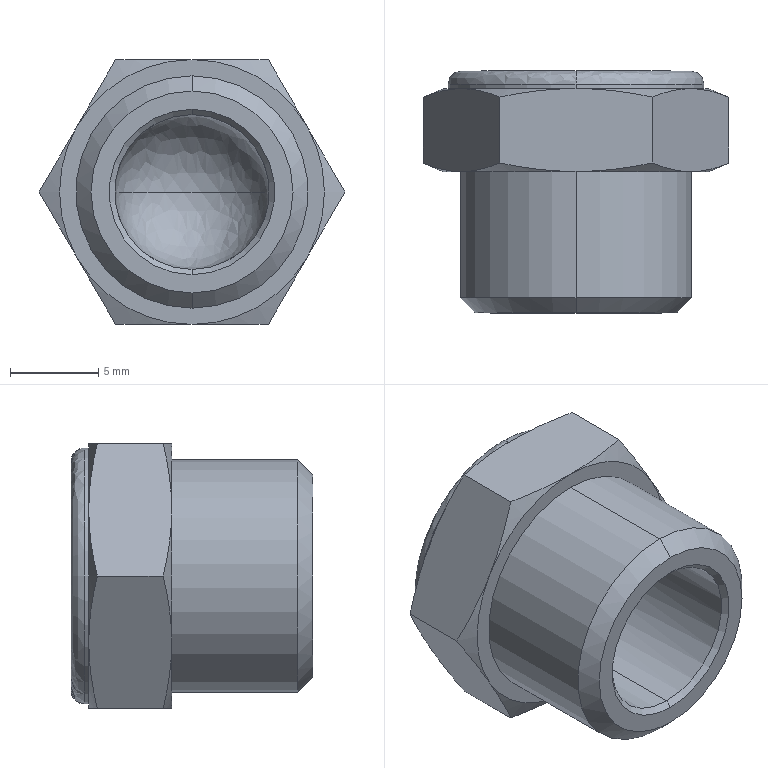Part | STEP file | 11-bslm02-V2.0-V2.011 | 1 solid | 39 faces | box 17.321 x 13.7 x 15 mm | volume 1416 mm3 | cone 16 | plane 11 | cylinder 8 | spline 4 | commonest cylinder face diameters 8.771 x2 11 x2 13.157 x2 14.5 x2
STEP:
#1=CARTESIAN_POINT('',(0.,8.314,-4.386));
#2=VERTEX_POINT('',#1);
#3=CARTESIAN_POINT('',(4.386,8.314,0.));
#4=VERTEX_POINT('',#3);
#5=CARTESIAN_POINT('',(0.,8.314,0.));
#6=DIRECTION('',(0.,-1.,0.));
#7=DIRECTION('',(0.,0.,-1.));
#8=AXIS2_PLACEMENT_3D('',#5,#6,#7);
#9=CIRCLE('',#8,4.386);
#10=EDGE_CURVE('',#2,#4,#9,.T.);
#11=ORIENTED_EDGE('',*,*,#10,.T.);
#12=CARTESIAN_POINT('',(-4.386,8.314,0.));
#13=VERTEX_POINT('',#12);
#14=CARTESIAN_POINT('',(0.,8.314,0.));
#15=DIRECTION('',(0.,0.,1.));
#16=DIRECTION('',(1.,0.,0.));
#17=AXIS2_PLACEMENT_3D('',#14,#15,#16);
#18=CIRCLE('',#17,4.386);
#19=EDGE_CURVE('',#4,#13,#18,.T.);
#20=ORIENTED_EDGE('',*,*,#19,.T.);
#21=CARTESIAN_POINT('',(0.,8.314,0.));
#22=DIRECTION('',(0.,-1.,0.));
#23=DIRECTION('',(0.,0.,-1.));
#24=AXIS2_PLACEMENT_3D('',#21,#22,#23);
#25=CIRCLE('',#24,4.386);
#26=EDGE_CURVE('',#13,#2,#25,.T.);
#27=ORIENTED_EDGE('',*,*,#26,.T.);
#28=EDGE_LOOP('',(#11,#20,#27));
#29=FACE_OUTER_BOUND('',#28,.T.);
#30=CARTESIAN_POINT('',(4.386,8.314,0.));
#31=CARTESIAN_POINT('',(4.386,8.314,0.));
#32=CARTESIAN_POINT('',(4.386,8.314,0.));
#33=CARTESIAN_POINT('',(4.386,8.314,0.));
#34=CARTESIAN_POINT('',(4.386,8.314,-8.771));
#35=CARTESIAN_POINT('',(4.386,13.452,-8.771));
#36=CARTESIAN_POINT('',(4.386,17.086,-5.138));
#37=CARTESIAN_POINT('',(4.386,17.086,0.));
#38=CARTESIAN_POINT('',(-4.386,8.314,-8.771));
#39=CARTESIAN_POINT('',(-4.386,13.452,-8.771));
#40=CARTESIAN_POINT('',(-4.386,17.086,-5.138));
#41=CARTESIAN_POINT('',(-4.386,17.086,0.));
#42=CARTESIAN_POINT('',(-4.386,8.314,0.));
#43=CARTESIAN_POINT('',(-4.386,8.314,0.));
#44=CARTESIAN_POINT('',(-4.386,8.314,0.));
#45=CARTESIAN_POINT('',(-4.386,8.314,0.));
#46=(BOUNDED_SURFACE()B_SPLINE_SURFACE(3,3,((#30,#31,#32,#33),(#34,#35,#36,#37),(#38,#39,#40,#41),(#42,#43,#44,#45)),.UNSPECIFIED.,.F.,.F.,.T.)B_SPLINE_SURFACE_WITH_KNOTS((4,4),(4,4),(0.,1.),(0.,1.),.UNSPECIFIED.)GEOMETRIC_REPRESENTATION_ITEM()RATIONAL_B_SPLINE_SURFACE(((1.,0.8047,0.8047,1.),(0.3333,0.2682,0.2682,0.3333),(0.3333,0.2682,0.2682,0.3333),(1.,0.8047,0.8047,1.)))REPRESENTATION_ITEM('')SURFACE());
#47=ADVANCED_FACE('',(#29),#46,.F.);
#48=CARTESIAN_POINT('',(0.,13.7,6.5));
#49=VERTEX_POINT('',#48);
#50=CARTESIAN_POINT('',(0.,13.7,-6.5));
#51=VERTEX_POINT('',#50);
#52=CARTESIAN_POINT('',(0.,13.7,6.5));
#53=CARTESIAN_POINT('',(-13.,13.7,6.5));
#54=CARTESIAN_POINT('',(-13.,13.7,-6.5));
#55=CARTESIAN_POINT('',(0.,13.7,-6.5));
#56=(BOUNDED_CURVE()B_SPLINE_CURVE(3,(#52,#53,#54,#55),.UNSPECIFIED.,.F.,.F.)B_SPLINE_CURVE_WITH_KNOTS((4,4),(0.,1.),.UNSPECIFIED.)CURVE()GEOMETRIC_REPRESENTATION_ITEM()RATIONAL_B_SPLINE_CURVE((1.,0.3333,0.3333,1.))REPRESENTATION_ITEM(''));
#57=EDGE_CURVE('',#49,#51,#56,.T.);
#58=ORIENTED_EDGE('',*,*,#57,.T.);
#59=CARTESIAN_POINT('',(0.,12.95,-7.25));
#60=VERTEX_POINT('',#59);
#61=CARTESIAN_POINT('',(0.,12.95,-6.5));
#62=DIRECTION('',(-1.,0.,0.));
#63=DIRECTION('',(0.,0.,-1.));
#64=AXIS2_PLACEMENT_3D('',#61,#62,#63);
#65=CIRCLE('',#64,0.75);
#66=EDGE_CURVE('',#51,#60,#65,.T.);
#67=ORIENTED_EDGE('',*,*,#66,.T.);
#68=CARTESIAN_POINT('',(0.,12.95,7.25));
#69=VERTEX_POINT('',#68);
#70=CARTESIAN_POINT('',(0.,12.95,0.));
#71=DIRECTION('',(0.,-1.,0.));
#72=DIRECTION('',(0.,0.,-1.));
#73=AXIS2_PLACEMENT_3D('',#70,#71,#72);
#74=CIRCLE('',#73,7.25);
#75=EDGE_CURVE('',#69,#60,#74,.T.);
#76=ORIENTED_EDGE('',*,*,#75,.F.);
#77=CARTESIAN_POINT('',(0.,12.95,6.5));
#78=DIRECTION('',(1.,0.,0.));
#79=DIRECTION('',(0.,0.,1.));
#80=AXIS2_PLACEMENT_3D('',#77,#78,#79);
#81=CIRCLE('',#80,0.75);
#82=EDGE_CURVE('',#49,#69,#81,.T.);
#83=ORIENTED_EDGE('',*,*,#82,.F.);
#84=EDGE_LOOP('',(#58,#67,#76,#83));
#85=FACE_OUTER_BOUND('',#84,.T.);
#86=CARTESIAN_POINT('',(0.,13.7,-6.5));
#87=CARTESIAN_POINT('',(-13.,13.7,-6.5));
#88=CARTESIAN_POINT('',(-13.,13.7,6.5));
#89=CARTESIAN_POINT('',(0.,13.7,6.5));
#90=CARTESIAN_POINT('',(0.,13.7,-6.939));
#91=CARTESIAN_POINT('',(-13.879,13.7,-6.939));
#92=CARTESIAN_POINT('',(-13.879,13.7,6.939));
#93=CARTESIAN_POINT('',(0.,13.7,6.939));
#94=CARTESIAN_POINT('',(0.,13.389,-7.25));
#95=CARTESIAN_POINT('',(-14.5,13.389,-7.25));
#96=CARTESIAN_POINT('',(-14.5,13.389,7.25));
#97=CARTESIAN_POINT('',(0.,13.389,7.25));
#98=CARTESIAN_POINT('',(0.,12.95,-7.25));
#99=CARTESIAN_POINT('',(-14.5,12.95,-7.25));
#100=CARTESIAN_POINT('',(-14.5,12.95,7.25));
#101=CARTESIAN_POINT('',(0.,12.95,7.25));
#102=(BOUNDED_SURFACE()B_SPLINE_SURFACE(3,3,((#86,#87,#88,#89),(#90,#91,#92,#93),(#94,#95,#96,#97),(#98,#99,#100,#101)),.UNSPECIFIED.,.F.,.F.,.F.)B_SPLINE_SURFACE_WITH_KNOTS((4,4),(4,4),(0.,1.),(0.,1.),.UNSPECIFIED.)GEOMETRIC_REPRESENTATION_ITEM()RATIONAL_B_SPLINE_SURFACE(((1.,0.3333,0.3333,1.),(0.8047,0.2682,0.2682,0.8047),(0.8047,0.2682,0.2682,0.8047),(1.,0.3333,0.3333,1.)))REPRESENTATION_ITEM('')SURFACE());
#103=ADVANCED_FACE('',(#85),#102,.T.);
#104=CARTESIAN_POINT('',(0.,8.,-6.579));
#105=VERTEX_POINT('',#104);
#106=CARTESIAN_POINT('',(0.,8.,6.579));
#107=VERTEX_POINT('',#106);
#108=CARTESIAN_POINT('',(0.,8.,0.));
#109=DIRECTION('',(0.,-1.,0.));
#110=DIRECTION('',(0.,0.,-1.));
#111=AXIS2_PLACEMENT_3D('',#108,#109,#110);
#112=CIRCLE('',#111,6.579);
#113=EDGE_CURVE('',#105,#107,#112,.T.);
#114=ORIENTED_EDGE('',*,*,#113,.T.);
#115=CARTESIAN_POINT('',(0.,0.856,6.578));
#116=VERTEX_POINT('',#115);
#117=CARTESIAN_POINT('',(0.,4.428,6.579));
#118=DIRECTION('',(0.,-1.,0.));
#119=VECTOR('',#118,1000.);
#120=LINE('',#117,#119);
#121=EDGE_CURVE('',#107,#116,#120,.T.);
#122=ORIENTED_EDGE('',*,*,#121,.T.);
#123=CARTESIAN_POINT('',(0.,0.856,-6.578));
#124=VERTEX_POINT('',#123);
#125=CARTESIAN_POINT('',(0.,0.856,0.));
#126=DIRECTION('',(0.,1.,0.));
#127=DIRECTION('',(0.,0.,-1.));
#128=AXIS2_PLACEMENT_3D('',#125,#126,#127);
#129=CIRCLE('',#128,6.579);
#130=EDGE_CURVE('',#116,#124,#129,.T.);
#131=ORIENTED_EDGE('',*,*,#130,.T.);
#132=CARTESIAN_POINT('',(0.,4.428,-6.579));
#133=DIRECTION('',(0.,-1.,0.));
#134=VECTOR('',#133,1000.);
#135=LINE('',#132,#134);
#136=EDGE_CURVE('',#105,#124,#135,.T.);
#137=ORIENTED_EDGE('',*,*,#136,.F.);
#138=EDGE_LOOP('',(#114,#122,#131,#137));
#139=FACE_OUTER_BOUND('',#138,.T.);
#140=CARTESIAN_POINT('',(0.,4.428,0.));
#141=DIRECTION('',(0.,-1.,0.));
#142=DIRECTION('',(0.,0.,-1.));
#143=AXIS2_PLACEMENT_3D('',#140,#141,#142);
#144=CYLINDRICAL_SURFACE('',#143,6.579);
#145=ADVANCED_FACE('',(#139),#144,.T.);
#146=CARTESIAN_POINT('',(0.,0.,5.722));
#147=VERTEX_POINT('',#146);
#148=CARTESIAN_POINT('',(0.,0.,-5.722));
#149=VERTEX_POINT('',#148);
#150=CARTESIAN_POINT('',(0.,0.,0.));
#151=DIRECTION('',(0.,1.,0.));
#152=DIRECTION('',(0.,0.,1.));
#153=AXIS2_PLACEMENT_3D('',#150,#151,#152);
#154=CIRCLE('',#153,5.722);
#155=EDGE_CURVE('',#147,#149,#154,.T.);
#156=ORIENTED_EDGE('',*,*,#155,.T.);
#157=CARTESIAN_POINT('',(0.,0.856,-6.578));
#158=DIRECTION('',(0.,0.7071,-0.7071));
#159=VECTOR('',#158,1000.);
#160=LINE('',#157,#159);
#161=EDGE_CURVE('',#149,#124,#160,.T.);
#162=ORIENTED_EDGE('',*,*,#161,.T.);
#163=ORIENTED_EDGE('',*,*,#130,.F.);
#164=CARTESIAN_POINT('',(0.,0.856,6.578));
#165=DIRECTION('',(0.,0.7071,0.7071));
#166=VECTOR('',#165,1000.);
#167=LINE('',#164,#166);
#168=EDGE_CURVE('',#147,#116,#167,.T.);
#169=ORIENTED_EDGE('',*,*,#168,.F.);
#170=EDGE_LOOP('',(#156,#162,#163,#169));
#171=FACE_OUTER_BOUND('',#170,.T.);
#172=CARTESIAN_POINT('',(0.,0.856,0.));
#173=DIRECTION('',(0.,1.,0.));
#174=DIRECTION('',(0.,0.,1.));
#175=AXIS2_PLACEMENT_3D('',#172,#173,#174);
#176=CONICAL_SURFACE('',#175,6.578,0.7854);
#177=ADVANCED_FACE('',(#171),#176,.T.);
#178=CARTESIAN_POINT('',(0.,0.3,4.386));
#179=VERTEX_POINT('',#178);
#180=CARTESIAN_POINT('',(0.,0.3,-4.386));
#181=VERTEX_POINT('',#180);
#182=CARTESIAN_POINT('',(0.,0.3,0.));
#183=DIRECTION('',(0.,-1.,0.));
#184=DIRECTION('',(1.,0.,0.));
#185=AXIS2_PLACEMENT_3D('',#182,#183,#184);
#186=CIRCLE('',#185,4.386);
#187=EDGE_CURVE('',#179,#181,#186,.T.);
#188=ORIENTED_EDGE('',*,*,#187,.F.);
#189=CARTESIAN_POINT('',(0.,0.,4.686));
#190=VERTEX_POINT('',#189);
#191=CARTESIAN_POINT('',(0.,0.,4.686));
#192=DIRECTION('',(0.,-0.7071,0.7071));
#193=VECTOR('',#192,1000.);
#194=LINE('',#191,#193);
#195=EDGE_CURVE('',#179,#190,#194,.T.);
#196=ORIENTED_EDGE('',*,*,#195,.T.);
#197=CARTESIAN_POINT('',(0.,0.,-4.686));
#198=VERTEX_POINT('',#197);
#199=CARTESIAN_POINT('',(0.,0.,0.));
#200=DIRECTION('',(0.,1.,0.));
#201=DIRECTION('',(0.,0.,-1.));
#202=AXIS2_PLACEMENT_3D('',#199,#200,#201);
#203=CIRCLE('',#202,4.686);
#204=EDGE_CURVE('',#198,#190,#203,.T.);
#205=ORIENTED_EDGE('',*,*,#204,.F.);
#206=CARTESIAN_POINT('',(0.,0.,-4.686));
#207=DIRECTION('',(0.,-0.7071,-0.7071));
#208=VECTOR('',#207,1000.);
#209=LINE('',#206,#208);
#210=EDGE_CURVE('',#181,#198,#209,.T.);
#211=ORIENTED_EDGE('',*,*,#210,.F.);
#212=EDGE_LOOP('',(#188,#196,#205,#211));
#213=FACE_OUTER_BOUND('',#212,.T.);
#214=CARTESIAN_POINT('',(0.,0.,0.));
#215=DIRECTION('',(0.,-1.,0.));
#216=DIRECTION('',(0.,0.,-1.));
#217=AXIS2_PLACEMENT_3D('',#214,#215,#216);
#218=CONICAL_SURFACE('',#217,4.686,0.7854);
#219=ADVANCED_FACE('',(#213),#218,.F.);
#220=CARTESIAN_POINT('',(0.,8.314,4.386));
#221=VERTEX_POINT('',#220);
#222=CARTESIAN_POINT('',(0.,8.314,0.));
#223=DIRECTION('',(0.,-1.,0.));
#224=DIRECTION('',(0.,0.,-1.));
#225=AXIS2_PLACEMENT_3D('',#222,#223,#224);
#226=CIRCLE('',#225,4.386);
#227=EDGE_CURVE('',#221,#13,#226,.T.);
#228=ORIENTED_EDGE('',*,*,#227,.F.);
#229=CARTESIAN_POINT('',(0.,4.307,4.386));
#230=DIRECTION('',(0.,-1.,0.));
#231=VECTOR('',#230,1000.);
#232=LINE('',#229,#231);
#233=EDGE_CURVE('',#221,#179,#232,.T.);
#234=ORIENTED_EDGE('',*,*,#233,.T.);
#235=ORIENTED_EDGE('',*,*,#187,.T.);
#236=CARTESIAN_POINT('',(0.,4.307,-4.386));
#237=DIRECTION('',(0.,-1.,0.));
#238=VECTOR('',#237,1000.);
#239=LINE('',#236,#238);
#240=EDGE_CURVE('',#2,#181,#239,.T.);
#241=ORIENTED_EDGE('',*,*,#240,.F.);
#242=ORIENTED_EDGE('',*,*,#26,.F.);
#243=EDGE_LOOP('',(#228,#234,#235,#241,#242));
#244=FACE_OUTER_BOUND('',#243,.T.);
#245=CARTESIAN_POINT('',(0.,4.307,0.));
#246=DIRECTION('',(0.,-1.,0.));
#247=DIRECTION('',(0.,0.,-1.));
#248=AXIS2_PLACEMENT_3D('',#245,#246,#247);
#249=CYLINDRICAL_SURFACE('',#248,4.386);
#250=ADVANCED_FACE('',(#244),#249,.F.);
#251=CARTESIAN_POINT('',(0.,12.95,0.));
#252=DIRECTION('',(0.,-1.,0.));
#253=DIRECTION('',(0.,0.,-1.));
#254=AXIS2_PLACEMENT_3D('',#251,#252,#253);
#255=CIRCLE('',#254,7.25);
#256=EDGE_CURVE('',#60,#69,#255,.T.);
#257=ORIENTED_EDGE('',*,*,#256,.T.);
#258=CARTESIAN_POINT('',(0.,12.7,7.25));
#259=VERTEX_POINT('',#258);
#260=CARTESIAN_POINT('',(0.,12.825,7.25));
#261=DIRECTION('',(0.,-1.,0.));
#262=VECTOR('',#261,1000.);
#263=LINE('',#260,#262);
#264=EDGE_CURVE('',#69,#259,#263,.T.);
#265=ORIENTED_EDGE('',*,*,#264,.T.);
#266=CARTESIAN_POINT('',(0.,12.7,-7.25));
#267=VERTEX_POINT('',#266);
#268=CARTESIAN_POINT('',(0.,12.7,0.));
#269=DIRECTION('',(0.,-1.,0.));
#270=DIRECTION('',(0.,0.,-1.));
#271=AXIS2_PLACEMENT_3D('',#268,#269,#270);
#272=CIRCLE('',#271,7.25);
#273=EDGE_CURVE('',#267,#259,#272,.T.);
#274=ORIENTED_EDGE('',*,*,#273,.F.);
#275=CARTESIAN_POINT('',(0.,12.825,-7.25));
#276=DIRECTION('',(0.,-1.,0.));
#277=VECTOR('',#276,1000.);
#278=LINE('',#275,#277);
#279=EDGE_CURVE('',#60,#267,#278,.T.);
#280=ORIENTED_EDGE('',*,*,#279,.F.);
#281=EDGE_LOOP('',(#257,#265,#274,#280));
#282=FACE_OUTER_BOUND('',#281,.T.);
#283=CARTESIAN_POINT('',(0.,12.825,0.));
#284=DIRECTION('',(0.,-1.,0.));
#285=DIRECTION('',(0.,0.,-1.));
#286=AXIS2_PLACEMENT_3D('',#283,#284,#285);
#287=CYLINDRICAL_SURFACE('',#286,7.25);
#288=ADVANCED_FACE('',(#282),#287,.T.);
#289=CARTESIAN_POINT('',(0.,13.7,5.5));
#290=VERTEX_POINT('',#289);
#291=CARTESIAN_POINT('',(0.,13.7,-5.5));
#292=VERTEX_POINT('',#291);
#293=CARTESIAN_POINT('',(0.,13.7,0.));
#294=DIRECTION('',(0.,-1.,0.));
#295=DIRECTION('',(0.,0.,-1.));
#296=AXIS2_PLACEMENT_3D('',#293,#294,#295);
#297=CIRCLE('',#296,5.5);
#298=EDGE_CURVE('',#290,#292,#297,.T.);
#299=ORIENTED_EDGE('',*,*,#298,.F.);
#300=CARTESIAN_POINT('',(0.,13.2,5.5));
#301=VERTEX_POINT('',#300);
#302=CARTESIAN_POINT('',(0.,13.45,5.5));
#303=DIRECTION('',(0.,-1.,0.));
#304=VECTOR('',#303,1000.);
#305=LINE('',#302,#304);
#306=EDGE_CURVE('',#290,#301,#305,.T.);
#307=ORIENTED_EDGE('',*,*,#306,.T.);
#308=CARTESIAN_POINT('',(0.,13.2,-5.5));
#309=VERTEX_POINT('',#308);
#310=CARTESIAN_POINT('',(0.,13.2,0.));
#311=DIRECTION('',(0.,1.,0.));
#312=DIRECTION('',(0.,0.,-1.));
#313=AXIS2_PLACEMENT_3D('',#310,#311,#312);
#314=CIRCLE('',#313,5.5);
#315=EDGE_CURVE('',#309,#301,#314,.T.);
#316=ORIENTED_EDGE('',*,*,#315,.F.);
#317=CARTESIAN_POINT('',(0.,13.45,-5.5));
#318=DIRECTION('',(0.,-1.,0.));
#319=VECTOR('',#318,1000.);
#320=LINE('',#317,#319);
#321=EDGE_CURVE('',#292,#309,#320,.T.);
#322=ORIENTED_EDGE('',*,*,#321,.F.);
#323=EDGE_LOOP('',(#299,#307,#316,#322));
#324=FACE_OUTER_BOUND('',#323,.T.);
#325=CARTESIAN_POINT('',(0.,13.45,0.));
#326=DIRECTION('',(0.,-1.,0.));
#327=DIRECTION('',(0.,0.,-1.));
#328=AXIS2_PLACEMENT_3D('',#325,#326,#327);
#329=CYLINDRICAL_SURFACE('',#328,5.5);
#330=ADVANCED_FACE('',(#324),#329,.F.);
#331=ORIENTED_EDGE('',*,*,#121,.F.);
#332=CARTESIAN_POINT('',(0.,8.,0.));
#333=DIRECTION('',(0.,-1.,0.));
#334=DIRECTION('',(0.,0.,-1.));
#335=AXIS2_PLACEMENT_3D('',#332,#333,#334);
#336=CIRCLE('',#335,6.579);
#337=EDGE_CURVE('',#107,#105,#336,.T.);
#338=ORIENTED_EDGE('',*,*,#337,.T.);
#339=ORIENTED_EDGE('',*,*,#136,.T.);
#340=CARTESIAN_POINT('',(0.,0.856,0.));
#341=DIRECTION('',(0.,1.,0.));
#342=DIRECTION('',(0.,0.,-1.));
#343=AXIS2_PLACEMENT_3D('',#340,#341,#342);
#344=CIRCLE('',#343,6.579);
#345=EDGE_CURVE('',#124,#116,#344,.T.);
#346=ORIENTED_EDGE('',*,*,#345,.T.);
#347=EDGE_LOOP('',(#331,#338,#339,#346));
#348=FACE_OUTER_BOUND('',#347,.T.);
#349=CARTESIAN_POINT('',(0.,4.428,0.));
#350=DIRECTION('',(0.,-1.,0.));
#351=DIRECTION('',(0.,0.,-1.));
#352=AXIS2_PLACEMENT_3D('',#349,#350,#351);
#353=CYLINDRICAL_SURFACE('',#352,6.579);
#354=ADVANCED_FACE('',(#348),#353,.T.);
#355=ORIENTED_EDGE('',*,*,#113,.F.);
#356=ORIENTED_EDGE('',*,*,#337,.F.);
#357=EDGE_LOOP('',(#355,#356));
#358=FACE_BOUND('',#357,.T.);
#359=CARTESIAN_POINT('',(0.,8.,-7.5));
#360=VERTEX_POINT('',#359);
#361=CARTESIAN_POINT('',(6.495,8.,-3.75));
#362=VERTEX_POINT('',#361);
#363=CARTESIAN_POINT('',(0.,8.,0.));
#364=DIRECTION('',(0.,-1.,0.));
#365=DIRECTION('',(0.,0.,1.));
#366=AXIS2_PLACEMENT_3D('',#363,#364,#365);
#367=CIRCLE('',#366,7.5);
#368=EDGE_CURVE('',#360,#362,#367,.T.);
#369=ORIENTED_EDGE('',*,*,#368,.T.);
#370=CARTESIAN_POINT('',(6.495,8.,3.75));
#371=VERTEX_POINT('',#370);
#372=CARTESIAN_POINT('',(0.,8.,0.));
#373=DIRECTION('',(0.,-1.,0.));
#374=DIRECTION('',(0.,0.,1.));
#375=AXIS2_PLACEMENT_3D('',#372,#373,#374);
#376=CIRCLE('',#375,7.5);
#377=EDGE_CURVE('',#362,#371,#376,.T.);
#378=ORIENTED_EDGE('',*,*,#377,.T.);
#379=CARTESIAN_POINT('',(0.,8.,7.5));
#380=VERTEX_POINT('',#379);
#381=CARTESIAN_POINT('',(0.,8.,0.));
#382=DIRECTION('',(0.,-1.,0.));
#383=DIRECTION('',(0.,0.,1.));
#384=AXIS2_PLACEMENT_3D('',#381,#382,#383);
#385=CIRCLE('',#384,7.5);
#386=EDGE_CURVE('',#371,#380,#385,.T.);
#387=ORIENTED_EDGE('',*,*,#386,.T.);
#388=CARTESIAN_POINT('',(-6.495,8.,3.75));
#389=VERTEX_POINT('',#388);
#390=CARTESIAN_POINT('',(0.,8.,0.));
#391=DIRECTION('',(0.,-1.,0.));
#392=DIRECTION('',(0.,0.,1.));
#393=AXIS2_PLACEMENT_3D('',#390,#391,#392);
#394=CIRCLE('',#393,7.5);
#395=EDGE_CURVE('',#380,#389,#394,.T.);
#396=ORIENTED_EDGE('',*,*,#395,.T.);
#397=CARTESIAN_POINT('',(-6.495,8.,-3.75));
#398=VERTEX_POINT('',#397);
#399=CARTESIAN_POINT('',(0.,8.,0.));
#400=DIRECTION('',(0.,-1.,0.));
#401=DIRECTION('',(0.,0.,1.));
#402=AXIS2_PLACEMENT_3D('',#399,#400,#401);
#403=CIRCLE('',#402,7.5);
#404=EDGE_CURVE('',#389,#398,#403,.T.);
#405=ORIENTED_EDGE('',*,*,#404,.T.);
#406=CARTESIAN_POINT('',(0.,8.,0.));
#407=DIRECTION('',(0.,-1.,0.));
#408=DIRECTION('',(0.,0.,1.));
#409=AXIS2_PLACEMENT_3D('',#406,#407,#408);
#410=CIRCLE('',#409,7.5);
#411=EDGE_CURVE('',#398,#360,#410,.T.);
#412=ORIENTED_EDGE('',*,*,#411,.T.);
#413=EDGE_LOOP('',(#369,#378,#387,#396,#405,#412));
#414=FACE_OUTER_BOUND('',#413,.T.);
#415=CARTESIAN_POINT('',(7.039,8.,0.));
#416=DIRECTION('',(0.,-1.,0.));
#417=DIRECTION('',(0.,0.,-1.));
#418=AXIS2_PLACEMENT_3D('',#415,#416,#417);
#419=PLANE('',#418);
#420=ADVANCED_FACE('',(#358,#414),#419,.T.);
#421=ORIENTED_EDGE('',*,*,#161,.F.);
#422=CARTESIAN_POINT('',(0.,0.,0.));
#423=DIRECTION('',(0.,1.,0.));
#424=DIRECTION('',(0.,0.,1.));
#425=AXIS2_PLACEMENT_3D('',#422,#423,#424);
#426=CIRCLE('',#425,5.722);
#427=EDGE_CURVE('',#149,#147,#426,.T.);
#428=ORIENTED_EDGE('',*,*,#427,.T.);
#429=ORIENTED_EDGE('',*,*,#168,.T.);
#430=ORIENTED_EDGE('',*,*,#345,.F.);
#431=EDGE_LOOP('',(#421,#428,#429,#430));
#432=FACE_OUTER_BOUND('',#431,.T.);
#433=CARTESIAN_POINT('',(0.,0.856,0.));
#434=DIRECTION('',(0.,1.,0.));
#435=DIRECTION('',(0.,0.,1.));
#436=AXIS2_PLACEMENT_3D('',#433,#434,#435);
#437=CONICAL_SURFACE('',#436,6.578,0.7854);
#438=ADVANCED_FACE('',(#432),#437,.T.);
#439=ORIENTED_EDGE('',*,*,#377,.F.);
#440=CARTESIAN_POINT('',(8.66,8.481,0.));
#441=VERTEX_POINT('',#440);
#442=CARTESIAN_POINT('',(6.495,8.,-3.75));
#443=CARTESIAN_POINT('',(6.86,8.,-3.117));
#444=CARTESIAN_POINT('',(7.223,8.045,-2.489));
#445=CARTESIAN_POINT('',(7.945,8.212,-1.24));
#446=CARTESIAN_POINT('',(8.303,8.333,-0.6185));
#447=CARTESIAN_POINT('',(8.66,8.481,0.));
#448=B_SPLINE_CURVE_WITH_KNOTS('',3,(#442,#443,#444,#445,#446,#447),.UNSPECIFIED.,.F.,.F.,(4,2,4),(0.,0.002178,0.004357),.UNSPECIFIED.);
#449=EDGE_CURVE('',#362,#441,#448,.T.);
#450=ORIENTED_EDGE('',*,*,#449,.T.);
#451=CARTESIAN_POINT('',(8.66,8.481,0.));
#452=CARTESIAN_POINT('',(8.303,8.333,0.6185));
#453=CARTESIAN_POINT('',(7.945,8.212,1.24));
#454=CARTESIAN_POINT('',(7.223,8.045,2.489));
#455=CARTESIAN_POINT('',(6.86,8.,3.117));
#456=CARTESIAN_POINT('',(6.495,8.,3.75));
#457=B_SPLINE_CURVE_WITH_KNOTS('',3,(#451,#452,#453,#454,#455,#456),.UNSPECIFIED.,.F.,.F.,(4,2,4),(0.,0.002178,0.004357),.UNSPECIFIED.);
#458=EDGE_CURVE('',#441,#371,#457,.T.);
#459=ORIENTED_EDGE('',*,*,#458,.T.);
#460=EDGE_LOOP('',(#439,#450,#459));
#461=FACE_OUTER_BOUND('',#460,.T.);
#462=CARTESIAN_POINT('',(0.,8.483,0.));
#463=DIRECTION('',(0.,1.,0.));
#464=DIRECTION('',(0.,0.,1.));
#465=AXIS2_PLACEMENT_3D('',#462,#463,#464);
#466=CONICAL_SURFACE('',#465,8.667,1.178);
#467=ADVANCED_FACE('',(#461),#466,.T.);
#468=ORIENTED_EDGE('',*,*,#368,.F.);
#469=CARTESIAN_POINT('',(4.33,8.481,-7.5));
#470=VERTEX_POINT('',#469);
#471=CARTESIAN_POINT('',(0.,8.,-7.5));
#472=CARTESIAN_POINT('',(0.7306,8.,-7.5));
#473=CARTESIAN_POINT('',(1.456,8.045,-7.5));
#474=CARTESIAN_POINT('',(2.899,8.212,-7.5));
#475=CARTESIAN_POINT('',(3.616,8.333,-7.5));
#476=CARTESIAN_POINT('',(4.33,8.481,-7.5));
#477=B_SPLINE_CURVE_WITH_KNOTS('',3,(#471,#472,#473,#474,#475,#476),.UNSPECIFIED.,.F.,.F.,(4,2,4),(0.,0.002178,0.004357),.UNSPECIFIED.);
#478=EDGE_CURVE('',#360,#470,#477,.T.);
#479=ORIENTED_EDGE('',*,*,#478,.T.);
#480=CARTESIAN_POINT('',(4.33,8.481,-7.5));
#481=CARTESIAN_POINT('',(4.687,8.333,-6.882));
#482=CARTESIAN_POINT('',(5.046,8.212,-6.26));
#483=CARTESIAN_POINT('',(5.767,8.045,-5.011));
#484=CARTESIAN_POINT('',(6.13,8.,-4.383));
#485=CARTESIAN_POINT('',(6.495,8.,-3.75));
#486=B_SPLINE_CURVE_WITH_KNOTS('',3,(#480,#481,#482,#483,#484,#485),.UNSPECIFIED.,.F.,.F.,(4,2,4),(0.,0.002178,0.004357),.UNSPECIFIED.);
#487=EDGE_CURVE('',#470,#362,#486,.T.);
#488=ORIENTED_EDGE('',*,*,#487,.T.);
#489=EDGE_LOOP('',(#468,#479,#488));
#490=FACE_OUTER_BOUND('',#489,.T.);
#491=CARTESIAN_POINT('',(0.,8.483,0.));
#492=DIRECTION('',(0.,1.,0.));
#493=DIRECTION('',(0.,0.,1.));
#494=AXIS2_PLACEMENT_3D('',#491,#492,#493);
#495=CONICAL_SURFACE('',#494,8.667,1.178);
#496=ADVANCED_FACE('',(#490),#495,.T.);
#497=CARTESIAN_POINT('',(-4.33,8.481,-7.5));
#498=VERTEX_POINT('',#497);
#499=CARTESIAN_POINT('',(-4.33,8.481,-7.5));
#500=CARTESIAN_POINT('',(-3.616,8.333,-7.5));
#501=CARTESIAN_POINT('',(-2.899,8.212,-7.5));
#502=CARTESIAN_POINT('',(-1.456,8.045,-7.5));
#503=CARTESIAN_POINT('',(-0.7306,8.,-7.5));
#504=CARTESIAN_POINT('',(0.,8.,-7.5));
#505=B_SPLINE_CURVE_WITH_KNOTS('',3,(#499,#500,#501,#502,#503,#504),.UNSPECIFIED.,.F.,.F.,(4,2,4),(0.,0.002178,0.004357),.UNSPECIFIED.);
#506=EDGE_CURVE('',#498,#360,#505,.T.);
#507=ORIENTED_EDGE('',*,*,#506,.T.);
#508=ORIENTED_EDGE('',*,*,#411,.F.);
#509=CARTESIAN_POINT('',(-6.495,8.,-3.75));
#510=CARTESIAN_POINT('',(-6.13,8.,-4.383));
#511=CARTESIAN_POINT('',(-5.767,8.045,-5.011));
#512=CARTESIAN_POINT('',(-5.046,8.212,-6.26));
#513=CARTESIAN_POINT('',(-4.687,8.333,-6.882));
#514=CARTESIAN_POINT('',(-4.33,8.481,-7.5));
#515=B_SPLINE_CURVE_WITH_KNOTS('',3,(#509,#510,#511,#512,#513,#514),.UNSPECIFIED.,.F.,.F.,(4,2,4),(0.,0.002178,0.004357),.UNSPECIFIED.);
#516=EDGE_CURVE('',#398,#498,#515,.T.);
#517=ORIENTED_EDGE('',*,*,#516,.T.);
#518=EDGE_LOOP('',(#507,#508,#517));
#519=FACE_OUTER_BOUND('',#518,.T.);
#520=CARTESIAN_POINT('',(0.,8.483,0.));
#521=DIRECTION('',(0.,1.,0.));
#522=DIRECTION('',(0.,0.,1.));
#523=AXIS2_PLACEMENT_3D('',#520,#521,#522);
#524=CONICAL_SURFACE('',#523,8.667,1.178);
#525=ADVANCED_FACE('',(#519),#524,.T.);
#526=CARTESIAN_POINT('',(-8.66,8.481,0.));
#527=VERTEX_POINT('',#526);
#528=CARTESIAN_POINT('',(-8.66,8.481,0.));
#529=CARTESIAN_POINT('',(-8.303,8.333,-0.6185));
#530=CARTESIAN_POINT('',(-7.945,8.212,-1.24));
#531=CARTESIAN_POINT('',(-7.223,8.045,-2.489));
#532=CARTESIAN_POINT('',(-6.86,8.,-3.117));
#533=CARTESIAN_POINT('',(-6.495,8.,-3.75));
#534=B_SPLINE_CURVE_WITH_KNOTS('',3,(#528,#529,#530,#531,#532,#533),.UNSPECIFIED.,.F.,.F.,(4,2,4),(0.,0.002178,0.004357),.UNSPECIFIED.);
#535=EDGE_CURVE('',#527,#398,#534,.T.);
#536=ORIENTED_EDGE('',*,*,#535,.T.);
#537=ORIENTED_EDGE('',*,*,#404,.F.);
#538=CARTESIAN_POINT('',(-6.495,8.,3.75));
#539=CARTESIAN_POINT('',(-6.86,8.,3.117));
#540=CARTESIAN_POINT('',(-7.223,8.045,2.489));
#541=CARTESIAN_POINT('',(-7.945,8.212,1.24));
#542=CARTESIAN_POINT('',(-8.303,8.333,0.6185));
#543=CARTESIAN_POINT('',(-8.66,8.481,0.));
#544=B_SPLINE_CURVE_WITH_KNOTS('',3,(#538,#539,#540,#541,#542,#543),.UNSPECIFIED.,.F.,.F.,(4,2,4),(0.,0.002178,0.004357),.UNSPECIFIED.);
#545=EDGE_CURVE('',#389,#527,#544,.T.);
#546=ORIENTED_EDGE('',*,*,#545,.T.);
#547=EDGE_LOOP('',(#536,#537,#546));
#548=FACE_OUTER_BOUND('',#547,.T.);
#549=CARTESIAN_POINT('',(0.,8.483,0.));
#550=DIRECTION('',(0.,1.,0.));
#551=DIRECTION('',(0.,0.,1.));
#552=AXIS2_PLACEMENT_3D('',#549,#550,#551);
#553=CONICAL_SURFACE('',#552,8.667,1.178);
#554=ADVANCED_FACE('',(#548),#553,.T.);
#555=CARTESIAN_POINT('',(-4.33,8.481,7.5));
#556=VERTEX_POINT('',#555);
#557=CARTESIAN_POINT('',(-4.33,8.481,7.5));
#558=CARTESIAN_POINT('',(-4.687,8.333,6.882));
#559=CARTESIAN_POINT('',(-5.046,8.212,6.26));
#560=CARTESIAN_POINT('',(-5.767,8.045,5.011));
#561=CARTESIAN_POINT('',(-6.13,8.,4.383));
#562=CARTESIAN_POINT('',(-6.495,8.,3.75));
#563=B_SPLINE_CURVE_WITH_KNOTS('',3,(#557,#558,#559,#560,#561,#562),.UNSPECIFIED.,.F.,.F.,(4,2,4),(0.,0.002178,0.004357),.UNSPECIFIED.);
#564=EDGE_CURVE('',#556,#389,#563,.T.);
#565=ORIENTED_EDGE('',*,*,#564,.T.);
#566=ORIENTED_EDGE('',*,*,#395,.F.);
#567=CARTESIAN_POINT('',(0.,8.,7.5));
#568=CARTESIAN_POINT('',(-0.7306,8.,7.5));
#569=CARTESIAN_POINT('',(-1.456,8.045,7.5));
#570=CARTESIAN_POINT('',(-2.899,8.212,7.5));
#571=CARTESIAN_POINT('',(-3.616,8.333,7.5));
#572=CARTESIAN_POINT('',(-4.33,8.481,7.5));
#573=B_SPLINE_CURVE_WITH_KNOTS('',3,(#567,#568,#569,#570,#571,#572),.UNSPECIFIED.,.F.,.F.,(4,2,4),(0.,0.002178,0.004357),.UNSPECIFIED.);
#574=EDGE_CURVE('',#380,#556,#573,.T.);
#575=ORIENTED_EDGE('',*,*,#574,.T.);
#576=EDGE_LOOP('',(#565,#566,#575));
#577=FACE_OUTER_BOUND('',#576,.T.);
#578=CARTESIAN_POINT('',(0.,8.483,0.));
#579=DIRECTION('',(0.,1.,0.));
#580=DIRECTION('',(0.,0.,1.));
#581=AXIS2_PLACEMENT_3D('',#578,#579,#580);
#582=CONICAL_SURFACE('',#581,8.667,1.178);
#583=ADVANCED_FACE('',(#577),#582,.T.);
#584=ORIENTED_EDGE('',*,*,#386,.F.);
#585=CARTESIAN_POINT('',(4.33,8.481,7.5));
#586=VERTEX_POINT('',#585);
#587=CARTESIAN_POINT('',(6.495,8.,3.75));
#588=CARTESIAN_POINT('',(6.13,8.,4.383));
#589=CARTESIAN_POINT('',(5.767,8.045,5.011));
#590=CARTESIAN_POINT('',(5.046,8.212,6.26));
#591=CARTESIAN_POINT('',(4.687,8.333,6.882));
#592=CARTESIAN_POINT('',(4.33,8.481,7.5));
#593=B_SPLINE_CURVE_WITH_KNOTS('',3,(#587,#588,#589,#590,#591,#592),.UNSPECIFIED.,.F.,.F.,(4,2,4),(0.,0.002178,0.004357),.UNSPECIFIED.);
#594=EDGE_CURVE('',#371,#586,#593,.T.);
#595=ORIENTED_EDGE('',*,*,#594,.T.);
#596=CARTESIAN_POINT('',(4.33,8.481,7.5));
#597=CARTESIAN_POINT('',(3.616,8.333,7.5));
#598=CARTESIAN_POINT('',(2.899,8.212,7.5));
#599=CARTESIAN_POINT('',(1.456,8.045,7.5));
#600=CARTESIAN_POINT('',(0.7306,8.,7.5));
#601=CARTESIAN_POINT('',(0.,8.,7.5));
#602=B_SPLINE_CURVE_WITH_KNOTS('',3,(#596,#597,#598,#599,#600,#601),.UNSPECIFIED.,.F.,.F.,(4,2,4),(0.,0.002178,0.004357),.UNSPECIFIED.);
#603=EDGE_CURVE('',#586,#380,#602,.T.);
#604=ORIENTED_EDGE('',*,*,#603,.T.);
#605=EDGE_LOOP('',(#584,#595,#604));
#606=FACE_OUTER_BOUND('',#605,.T.);
#607=CARTESIAN_POINT('',(0.,8.483,0.));
#608=DIRECTION('',(0.,1.,0.));
#609=DIRECTION('',(0.,0.,1.));
#610=AXIS2_PLACEMENT_3D('',#607,#608,#609);
#611=CONICAL_SURFACE('',#610,8.667,1.178);
#612=ADVANCED_FACE('',(#606),#611,.T.);
#613=ORIENTED_EDGE('',*,*,#204,.T.);
#614=CARTESIAN_POINT('',(0.,0.,0.));
#615=DIRECTION('',(0.,1.,0.));
#616=DIRECTION('',(0.,0.,-1.));
#617=AXIS2_PLACEMENT_3D('',#614,#615,#616);
#618=CIRCLE('',#617,4.686);
#619=EDGE_CURVE('',#190,#198,#618,.T.);
#620=ORIENTED_EDGE('',*,*,#619,.T.);
#621=EDGE_LOOP('',(#613,#620));
#622=FACE_BOUND('',#621,.T.);
#623=ORIENTED_EDGE('',*,*,#155,.F.);
#624=ORIENTED_EDGE('',*,*,#427,.F.);
#625=EDGE_LOOP('',(#623,#624));
#626=FACE_OUTER_BOUND('',#625,.T.);
#627=CARTESIAN_POINT('',(5.204,0.,0.));
#628=DIRECTION('',(0.,-1.,0.));
#629=DIRECTION('',(0.,0.,-1.));
#630=AXIS2_PLACEMENT_3D('',#627,#628,#629);
#631=PLANE('',#630);
#632=ADVANCED_FACE('',(#622,#626),#631,.T.);
#633=CARTESIAN_POINT('',(8.66,12.219,0.));
#634=VERTEX_POINT('',#633);
#635=CARTESIAN_POINT('',(8.66,0.,0.));
#636=DIRECTION('',(0.,1.,0.));
#637=VECTOR('',#636,1000.);
#638=LINE('',#635,#637);
#639=EDGE_CURVE('',#441,#634,#638,.T.);
#640=ORIENTED_EDGE('',*,*,#639,.F.);
#641=ORIENTED_EDGE('',*,*,#449,.F.);
#642=ORIENTED_EDGE('',*,*,#487,.F.);
#643=CARTESIAN_POINT('',(4.33,12.219,-7.5));
#644=VERTEX_POINT('',#643);
#645=CARTESIAN_POINT('',(4.33,0.,-7.5));
#646=DIRECTION('',(0.,-1.,0.));
#647=VECTOR('',#646,1000.);
#648=LINE('',#645,#647);
#649=EDGE_CURVE('',#644,#470,#648,.T.);
#650=ORIENTED_EDGE('',*,*,#649,.F.);
#651=CARTESIAN_POINT('',(6.495,12.7,-3.75));
#652=VERTEX_POINT('',#651);
#653=CARTESIAN_POINT('',(6.495,12.7,-3.75));
#654=CARTESIAN_POINT('',(6.13,12.7,-4.383));
#655=CARTESIAN_POINT('',(5.767,12.655,-5.011));
#656=CARTESIAN_POINT('',(5.046,12.488,-6.26));
#657=CARTESIAN_POINT('',(4.687,12.367,-6.882));
#658=CARTESIAN_POINT('',(4.33,12.219,-7.5));
#659=B_SPLINE_CURVE_WITH_KNOTS('',3,(#653,#654,#655,#656,#657,#658),.UNSPECIFIED.,.F.,.F.,(4,2,4),(0.,0.002178,0.004357),.UNSPECIFIED.);
#660=EDGE_CURVE('',#652,#644,#659,.T.);
#661=ORIENTED_EDGE('',*,*,#660,.F.);
#662=CARTESIAN_POINT('',(8.66,12.219,0.));
#663=CARTESIAN_POINT('',(8.303,12.367,-0.6185));
#664=CARTESIAN_POINT('',(7.945,12.488,-1.24));
#665=CARTESIAN_POINT('',(7.223,12.655,-2.489));
#666=CARTESIAN_POINT('',(6.86,12.7,-3.117));
#667=CARTESIAN_POINT('',(6.495,12.7,-3.75));
#668=B_SPLINE_CURVE_WITH_KNOTS('',3,(#662,#663,#664,#665,#666,#667),.UNSPECIFIED.,.F.,.F.,(4,2,4),(0.,0.002178,0.004357),.UNSPECIFIED.);
#669=EDGE_CURVE('',#634,#652,#668,.T.);
#670=ORIENTED_EDGE('',*,*,#669,.F.);
#671=EDGE_LOOP('',(#640,#641,#642,#650,#661,#670));
#672=FACE_OUTER_BOUND('',#671,.T.);
#673=CARTESIAN_POINT('',(8.66,0.,0.));
#674=DIRECTION('',(-0.866,0.,0.5));
#675=DIRECTION('',(0.5,0.,0.866));
#676=AXIS2_PLACEMENT_3D('',#673,#674,#675);
#677=PLANE('',#676);
#678=ADVANCED_FACE('',(#672),#677,.F.);
#679=ORIENTED_EDGE('',*,*,#649,.T.);
#680=ORIENTED_EDGE('',*,*,#478,.F.);
#681=ORIENTED_EDGE('',*,*,#506,.F.);
#682=CARTESIAN_POINT('',(-4.33,12.219,-7.5));
#683=VERTEX_POINT('',#682);
#684=CARTESIAN_POINT('',(-4.33,0.,-7.5));
#685=DIRECTION('',(0.,-1.,0.));
#686=VECTOR('',#685,1000.);
#687=LINE('',#684,#686);
#688=EDGE_CURVE('',#683,#498,#687,.T.);
#689=ORIENTED_EDGE('',*,*,#688,.F.);
#690=CARTESIAN_POINT('',(0.,12.7,-7.5));
#691=VERTEX_POINT('',#690);
#692=CARTESIAN_POINT('',(0.,12.7,-7.5));
#693=CARTESIAN_POINT('',(-0.7306,12.7,-7.5));
#694=CARTESIAN_POINT('',(-1.456,12.655,-7.5));
#695=CARTESIAN_POINT('',(-2.899,12.488,-7.5));
#696=CARTESIAN_POINT('',(-3.616,12.367,-7.5));
#697=CARTESIAN_POINT('',(-4.33,12.219,-7.5));
#698=B_SPLINE_CURVE_WITH_KNOTS('',3,(#692,#693,#694,#695,#696,#697),.UNSPECIFIED.,.F.,.F.,(4,2,4),(0.,0.002178,0.004357),.UNSPECIFIED.);
#699=EDGE_CURVE('',#691,#683,#698,.T.);
#700=ORIENTED_EDGE('',*,*,#699,.F.);
#701=CARTESIAN_POINT('',(4.33,12.219,-7.5));
#702=CARTESIAN_POINT('',(3.616,12.367,-7.5));
#703=CARTESIAN_POINT('',(2.899,12.488,-7.5));
#704=CARTESIAN_POINT('',(1.456,12.655,-7.5));
#705=CARTESIAN_POINT('',(0.7306,12.7,-7.5));
#706=CARTESIAN_POINT('',(0.,12.7,-7.5));
#707=B_SPLINE_CURVE_WITH_KNOTS('',3,(#701,#702,#703,#704,#705,#706),.UNSPECIFIED.,.F.,.F.,(4,2,4),(0.,0.002178,0.004357),.UNSPECIFIED.);
#708=EDGE_CURVE('',#644,#691,#707,.T.);
#709=ORIENTED_EDGE('',*,*,#708,.F.);
#710=EDGE_LOOP('',(#679,#680,#681,#689,#700,#709));
#711=FACE_OUTER_BOUND('',#710,.T.);
#712=CARTESIAN_POINT('',(4.33,0.,-7.5));
#713=DIRECTION('',(0.,0.,1.));
#714=DIRECTION('',(1.,0.,0.));
#715=AXIS2_PLACEMENT_3D('',#712,#713,#714);
#716=PLANE('',#715);
#717=ADVANCED_FACE('',(#711),#716,.F.);
#718=CARTESIAN_POINT('',(-6.495,12.7,-3.75));
#719=VERTEX_POINT('',#718);
#720=CARTESIAN_POINT('',(-4.33,12.219,-7.5));
#721=CARTESIAN_POINT('',(-4.687,12.367,-6.882));
#722=CARTESIAN_POINT('',(-5.046,12.488,-6.26));
#723=CARTESIAN_POINT('',(-5.767,12.655,-5.011));
#724=CARTESIAN_POINT('',(-6.13,12.7,-4.383));
#725=CARTESIAN_POINT('',(-6.495,12.7,-3.75));
#726=B_SPLINE_CURVE_WITH_KNOTS('',3,(#720,#721,#722,#723,#724,#725),.UNSPECIFIED.,.F.,.F.,(4,2,4),(0.,0.002178,0.004357),.UNSPECIFIED.);
#727=EDGE_CURVE('',#683,#719,#726,.T.);
#728=ORIENTED_EDGE('',*,*,#727,.F.);
#729=ORIENTED_EDGE('',*,*,#688,.T.);
#730=ORIENTED_EDGE('',*,*,#516,.F.);
#731=ORIENTED_EDGE('',*,*,#535,.F.);
#732=CARTESIAN_POINT('',(-8.66,12.219,0.));
#733=VERTEX_POINT('',#732);
#734=CARTESIAN_POINT('',(-8.66,0.,0.));
#735=DIRECTION('',(0.,-1.,0.));
#736=VECTOR('',#735,1000.);
#737=LINE('',#734,#736);
#738=EDGE_CURVE('',#733,#527,#737,.T.);
#739=ORIENTED_EDGE('',*,*,#738,.F.);
#740=CARTESIAN_POINT('',(-6.495,12.7,-3.75));
#741=CARTESIAN_POINT('',(-6.86,12.7,-3.117));
#742=CARTESIAN_POINT('',(-7.223,12.655,-2.489));
#743=CARTESIAN_POINT('',(-7.945,12.488,-1.24));
#744=CARTESIAN_POINT('',(-8.303,12.367,-0.6185));
#745=CARTESIAN_POINT('',(-8.66,12.219,0.));
#746=B_SPLINE_CURVE_WITH_KNOTS('',3,(#740,#741,#742,#743,#744,#745),.UNSPECIFIED.,.F.,.F.,(4,2,4),(0.,0.002178,0.004357),.UNSPECIFIED.);
#747=EDGE_CURVE('',#719,#733,#746,.T.);
#748=ORIENTED_EDGE('',*,*,#747,.F.);
#749=EDGE_LOOP('',(#728,#729,#730,#731,#739,#748));
#750=FACE_OUTER_BOUND('',#749,.T.);
#751=CARTESIAN_POINT('',(-4.33,0.,-7.5));
#752=DIRECTION('',(0.866,0.,0.5));
#753=DIRECTION('',(0.5,0.,-0.866));
#754=AXIS2_PLACEMENT_3D('',#751,#752,#753);
#755=PLANE('',#754);
#756=ADVANCED_FACE('',(#750),#755,.F.);
#757=CARTESIAN_POINT('',(-6.495,12.7,3.75));
#758=VERTEX_POINT('',#757);
#759=CARTESIAN_POINT('',(-8.66,12.219,0.));
#760=CARTESIAN_POINT('',(-8.303,12.367,0.6185));
#761=CARTESIAN_POINT('',(-7.945,12.488,1.24));
#762=CARTESIAN_POINT('',(-7.223,12.655,2.489));
#763=CARTESIAN_POINT('',(-6.86,12.7,3.117));
#764=CARTESIAN_POINT('',(-6.495,12.7,3.75));
#765=B_SPLINE_CURVE_WITH_KNOTS('',3,(#759,#760,#761,#762,#763,#764),.UNSPECIFIED.,.F.,.F.,(4,2,4),(0.,0.002178,0.004357),.UNSPECIFIED.);
#766=EDGE_CURVE('',#733,#758,#765,.T.);
#767=ORIENTED_EDGE('',*,*,#766,.F.);
#768=ORIENTED_EDGE('',*,*,#738,.T.);
#769=ORIENTED_EDGE('',*,*,#545,.F.);
#770=ORIENTED_EDGE('',*,*,#564,.F.);
#771=CARTESIAN_POINT('',(-4.33,12.219,7.5));
#772=VERTEX_POINT('',#771);
#773=CARTESIAN_POINT('',(-4.33,0.,7.5));
#774=DIRECTION('',(0.,-1.,0.));
#775=VECTOR('',#774,1000.);
#776=LINE('',#773,#775);
#777=EDGE_CURVE('',#772,#556,#776,.T.);
#778=ORIENTED_EDGE('',*,*,#777,.F.);
#779=CARTESIAN_POINT('',(-6.495,12.7,3.75));
#780=CARTESIAN_POINT('',(-6.13,12.7,4.383));
#781=CARTESIAN_POINT('',(-5.767,12.655,5.011));
#782=CARTESIAN_POINT('',(-5.046,12.488,6.26));
#783=CARTESIAN_POINT('',(-4.687,12.367,6.882));
#784=CARTESIAN_POINT('',(-4.33,12.219,7.5));
#785=B_SPLINE_CURVE_WITH_KNOTS('',3,(#779,#780,#781,#782,#783,#784),.UNSPECIFIED.,.F.,.F.,(4,2,4),(0.,0.002178,0.004357),.UNSPECIFIED.);
#786=EDGE_CURVE('',#758,#772,#785,.T.);
#787=ORIENTED_EDGE('',*,*,#786,.F.);
#788=EDGE_LOOP('',(#767,#768,#769,#770,#778,#787));
#789=FACE_OUTER_BOUND('',#788,.T.);
#790=CARTESIAN_POINT('',(-8.66,0.,0.));
#791=DIRECTION('',(0.866,0.,-0.5));
#792=DIRECTION('',(-0.5,0.,-0.866));
#793=AXIS2_PLACEMENT_3D('',#790,#791,#792);
#794=PLANE('',#793);
#795=ADVANCED_FACE('',(#789),#794,.F.);
#796=CARTESIAN_POINT('',(0.,12.7,7.5));
#797=VERTEX_POINT('',#796);
#798=CARTESIAN_POINT('',(-4.33,12.219,7.5));
#799=CARTESIAN_POINT('',(-3.616,12.367,7.5));
#800=CARTESIAN_POINT('',(-2.899,12.488,7.5));
#801=CARTESIAN_POINT('',(-1.456,12.655,7.5));
#802=CARTESIAN_POINT('',(-0.7306,12.7,7.5));
#803=CARTESIAN_POINT('',(0.,12.7,7.5));
#804=B_SPLINE_CURVE_WITH_KNOTS('',3,(#798,#799,#800,#801,#802,#803),.UNSPECIFIED.,.F.,.F.,(4,2,4),(0.,0.002178,0.004357),.UNSPECIFIED.);
#805=EDGE_CURVE('',#772,#797,#804,.T.);
#806=ORIENTED_EDGE('',*,*,#805,.F.);
#807=ORIENTED_EDGE('',*,*,#777,.T.);
#808=ORIENTED_EDGE('',*,*,#574,.F.);
#809=ORIENTED_EDGE('',*,*,#603,.F.);
#810=CARTESIAN_POINT('',(4.33,12.219,7.5));
#811=VERTEX_POINT('',#810);
#812=CARTESIAN_POINT('',(4.33,0.,7.5));
#813=DIRECTION('',(0.,-1.,0.));
#814=VECTOR('',#813,1000.);
#815=LINE('',#812,#814);
#816=EDGE_CURVE('',#811,#586,#815,.T.);
#817=ORIENTED_EDGE('',*,*,#816,.F.);
#818=CARTESIAN_POINT('',(0.,12.7,7.5));
#819=CARTESIAN_POINT('',(0.7306,12.7,7.5));
#820=CARTESIAN_POINT('',(1.456,12.655,7.5));
#821=CARTESIAN_POINT('',(2.899,12.488,7.5));
#822=CARTESIAN_POINT('',(3.616,12.367,7.5));
#823=CARTESIAN_POINT('',(4.33,12.219,7.5));
#824=B_SPLINE_CURVE_WITH_KNOTS('',3,(#818,#819,#820,#821,#822,#823),.UNSPECIFIED.,.F.,.F.,(4,2,4),(0.,0.002178,0.004357),.UNSPECIFIED.);
#825=EDGE_CURVE('',#797,#811,#824,.T.);
#826=ORIENTED_EDGE('',*,*,#825,.F.);
#827=EDGE_LOOP('',(#806,#807,#808,#809,#817,#826));
#828=FACE_OUTER_BOUND('',#827,.T.);
#829=CARTESIAN_POINT('',(-4.33,0.,7.5));
#830=DIRECTION('',(0.,0.,-1.));
#831=DIRECTION('',(-1.,0.,0.));
#832=AXIS2_PLACEMENT_3D('',#829,#830,#831);
#833=PLANE('',#832);
#834=ADVANCED_FACE('',(#828),#833,.F.);
#835=ORIENTED_EDGE('',*,*,#816,.T.);
#836=ORIENTED_EDGE('',*,*,#594,.F.);
#837=ORIENTED_EDGE('',*,*,#458,.F.);
#838=ORIENTED_EDGE('',*,*,#639,.T.);
#839=CARTESIAN_POINT('',(6.495,12.7,3.75));
#840=VERTEX_POINT('',#839);
#841=CARTESIAN_POINT('',(6.495,12.7,3.75));
#842=CARTESIAN_POINT('',(6.86,12.7,3.117));
#843=CARTESIAN_POINT('',(7.223,12.655,2.489));
#844=CARTESIAN_POINT('',(7.945,12.488,1.24));
#845=CARTESIAN_POINT('',(8.303,12.367,0.6185));
#846=CARTESIAN_POINT('',(8.66,12.219,0.));
#847=B_SPLINE_CURVE_WITH_KNOTS('',3,(#841,#842,#843,#844,#845,#846),.UNSPECIFIED.,.F.,.F.,(4,2,4),(0.,0.002178,0.004357),.UNSPECIFIED.);
#848=EDGE_CURVE('',#840,#634,#847,.T.);
#849=ORIENTED_EDGE('',*,*,#848,.F.);
#850=CARTESIAN_POINT('',(4.33,12.219,7.5));
#851=CARTESIAN_POINT('',(4.687,12.367,6.882));
#852=CARTESIAN_POINT('',(5.046,12.488,6.26));
#853=CARTESIAN_POINT('',(5.767,12.655,5.011));
#854=CARTESIAN_POINT('',(6.13,12.7,4.383));
#855=CARTESIAN_POINT('',(6.495,12.7,3.75));
#856=B_SPLINE_CURVE_WITH_KNOTS('',3,(#850,#851,#852,#853,#854,#855),.UNSPECIFIED.,.F.,.F.,(4,2,4),(0.,0.002178,0.004357),.UNSPECIFIED.);
#857=EDGE_CURVE('',#811,#840,#856,.T.);
#858=ORIENTED_EDGE('',*,*,#857,.F.);
#859=EDGE_LOOP('',(#835,#836,#837,#838,#849,#858));
#860=FACE_OUTER_BOUND('',#859,.T.);
#861=CARTESIAN_POINT('',(4.33,0.,7.5));
#862=DIRECTION('',(-0.866,0.,-0.5));
#863=DIRECTION('',(-0.5,0.,0.866));
#864=AXIS2_PLACEMENT_3D('',#861,#862,#863);
#865=PLANE('',#864);
#866=ADVANCED_FACE('',(#860),#865,.F.);
#867=ORIENTED_EDGE('',*,*,#195,.F.);
#868=CARTESIAN_POINT('',(0.,0.3,0.));
#869=DIRECTION('',(0.,-1.,0.));
#870=DIRECTION('',(1.,0.,0.));
#871=AXIS2_PLACEMENT_3D('',#868,#869,#870);
#872=CIRCLE('',#871,4.386);
#873=EDGE_CURVE('',#181,#179,#872,.T.);
#874=ORIENTED_EDGE('',*,*,#873,.F.);
#875=ORIENTED_EDGE('',*,*,#210,.T.);
#876=ORIENTED_EDGE('',*,*,#619,.F.);
#877=EDGE_LOOP('',(#867,#874,#875,#876));
#878=FACE_OUTER_BOUND('',#877,.T.);
#879=CARTESIAN_POINT('',(0.,0.,0.));
#880=DIRECTION('',(0.,-1.,0.));
#881=DIRECTION('',(0.,0.,-1.));
#882=AXIS2_PLACEMENT_3D('',#879,#880,#881);
#883=CONICAL_SURFACE('',#882,4.686,0.7854);
#884=ADVANCED_FACE('',(#878),#883,.F.);
#885=ORIENTED_EDGE('',*,*,#669,.T.);
#886=CARTESIAN_POINT('',(0.,12.7,0.));
#887=DIRECTION('',(0.,-1.,0.));
#888=DIRECTION('',(0.,0.,-1.));
#889=AXIS2_PLACEMENT_3D('',#886,#887,#888);
#890=CIRCLE('',#889,7.5);
#891=EDGE_CURVE('',#652,#840,#890,.T.);
#892=ORIENTED_EDGE('',*,*,#891,.T.);
#893=ORIENTED_EDGE('',*,*,#848,.T.);
#894=EDGE_LOOP('',(#885,#892,#893));
#895=FACE_OUTER_BOUND('',#894,.T.);
#896=CARTESIAN_POINT('',(0.,12.217,0.));
#897=DIRECTION('',(0.,-1.,0.));
#898=DIRECTION('',(0.,0.,-1.));
#899=AXIS2_PLACEMENT_3D('',#896,#897,#898);
#900=CONICAL_SURFACE('',#899,8.667,1.178);
#901=ADVANCED_FACE('',(#895),#900,.T.);
#902=ORIENTED_EDGE('',*,*,#708,.T.);
#903=CARTESIAN_POINT('',(0.,12.7,0.));
#904=DIRECTION('',(0.,-1.,0.));
#905=DIRECTION('',(0.,0.,-1.));
#906=AXIS2_PLACEMENT_3D('',#903,#904,#905);
#907=CIRCLE('',#906,7.5);
#908=EDGE_CURVE('',#691,#652,#907,.T.);
#909=ORIENTED_EDGE('',*,*,#908,.T.);
#910=ORIENTED_EDGE('',*,*,#660,.T.);
#911=EDGE_LOOP('',(#902,#909,#910));
#912=FACE_OUTER_BOUND('',#911,.T.);
#913=CARTESIAN_POINT('',(0.,12.217,0.));
#914=DIRECTION('',(0.,-1.,0.));
#915=DIRECTION('',(0.,0.,-1.));
#916=AXIS2_PLACEMENT_3D('',#913,#914,#915);
#917=CONICAL_SURFACE('',#916,8.667,1.178);
#918=ADVANCED_FACE('',(#912),#917,.T.);
#919=CARTESIAN_POINT('',(0.,12.7,0.));
#920=DIRECTION('',(0.,-1.,0.));
#921=DIRECTION('',(0.,0.,-1.));
#922=AXIS2_PLACEMENT_3D('',#919,#920,#921);
#923=CIRCLE('',#922,7.5);
#924=EDGE_CURVE('',#719,#691,#923,.T.);
#925=ORIENTED_EDGE('',*,*,#924,.T.);
#926=ORIENTED_EDGE('',*,*,#699,.T.);
#927=ORIENTED_EDGE('',*,*,#727,.T.);
#928=EDGE_LOOP('',(#925,#926,#927));
#929=FACE_OUTER_BOUND('',#928,.T.);
#930=CARTESIAN_POINT('',(0.,12.217,0.));
#931=DIRECTION('',(0.,-1.,0.));
#932=DIRECTION('',(0.,0.,-1.));
#933=AXIS2_PLACEMENT_3D('',#930,#931,#932);
#934=CONICAL_SURFACE('',#933,8.667,1.178);
#935=ADVANCED_FACE('',(#929),#934,.T.);
#936=CARTESIAN_POINT('',(0.,12.7,0.));
#937=DIRECTION('',(0.,-1.,0.));
#938=DIRECTION('',(0.,0.,-1.));
#939=AXIS2_PLACEMENT_3D('',#936,#937,#938);
#940=CIRCLE('',#939,7.5);
#941=EDGE_CURVE('',#758,#719,#940,.T.);
#942=ORIENTED_EDGE('',*,*,#941,.T.);
#943=ORIENTED_EDGE('',*,*,#747,.T.);
#944=ORIENTED_EDGE('',*,*,#766,.T.);
#945=EDGE_LOOP('',(#942,#943,#944));
#946=FACE_OUTER_BOUND('',#945,.T.);
#947=CARTESIAN_POINT('',(0.,12.217,0.));
#948=DIRECTION('',(0.,-1.,0.));
#949=DIRECTION('',(0.,0.,-1.));
#950=AXIS2_PLACEMENT_3D('',#947,#948,#949);
#951=CONICAL_SURFACE('',#950,8.667,1.178);
#952=ADVANCED_FACE('',(#946),#951,.T.);
#953=CARTESIAN_POINT('',(0.,12.7,0.));
#954=DIRECTION('',(0.,-1.,0.));
#955=DIRECTION('',(0.,0.,-1.));
#956=AXIS2_PLACEMENT_3D('',#953,#954,#955);
#957=CIRCLE('',#956,7.5);
#958=EDGE_CURVE('',#797,#758,#957,.T.);
#959=ORIENTED_EDGE('',*,*,#958,.T.);
#960=ORIENTED_EDGE('',*,*,#786,.T.);
#961=ORIENTED_EDGE('',*,*,#805,.T.);
#962=EDGE_LOOP('',(#959,#960,#961));
#963=FACE_OUTER_BOUND('',#962,.T.);
#964=CARTESIAN_POINT('',(0.,12.217,0.));
#965=DIRECTION('',(0.,-1.,0.));
#966=DIRECTION('',(0.,0.,-1.));
#967=AXIS2_PLACEMENT_3D('',#964,#965,#966);
#968=CONICAL_SURFACE('',#967,8.667,1.178);
#969=ADVANCED_FACE('',(#963),#968,.T.);
#970=ORIENTED_EDGE('',*,*,#857,.T.);
#971=CARTESIAN_POINT('',(0.,12.7,0.));
#972=DIRECTION('',(0.,-1.,0.));
#973=DIRECTION('',(0.,0.,-1.));
#974=AXIS2_PLACEMENT_3D('',#971,#972,#973);
#975=CIRCLE('',#974,7.5);
#976=EDGE_CURVE('',#840,#797,#975,.T.);
#977=ORIENTED_EDGE('',*,*,#976,.T.);
#978=ORIENTED_EDGE('',*,*,#825,.T.);
#979=EDGE_LOOP('',(#970,#977,#978));
#980=FACE_OUTER_BOUND('',#979,.T.);
#981=CARTESIAN_POINT('',(0.,12.217,0.));
#982=DIRECTION('',(0.,-1.,0.));
#983=DIRECTION('',(0.,0.,-1.));
#984=AXIS2_PLACEMENT_3D('',#981,#982,#983);
#985=CONICAL_SURFACE('',#984,8.667,1.178);
#986=ADVANCED_FACE('',(#980),#985,.T.);
#987=ORIENTED_EDGE('',*,*,#233,.F.);
#988=CARTESIAN_POINT('',(0.,8.314,0.));
#989=DIRECTION('',(0.,-1.,0.));
#990=DIRECTION('',(0.,0.,-1.));
#991=AXIS2_PLACEMENT_3D('',#988,#989,#990);
#992=CIRCLE('',#991,4.386);
#993=EDGE_CURVE('',#4,#221,#992,.T.);
#994=ORIENTED_EDGE('',*,*,#993,.F.);
#995=ORIENTED_EDGE('',*,*,#10,.F.);
#996=ORIENTED_EDGE('',*,*,#240,.T.);
#997=ORIENTED_EDGE('',*,*,#873,.T.);
#998=EDGE_LOOP('',(#987,#994,#995,#996,#997));
#999=FACE_OUTER_BOUND('',#998,.T.);
#1000=CARTESIAN_POINT('',(0.,4.307,0.));
#1001=DIRECTION('',(0.,-1.,0.));
#1002=DIRECTION('',(0.,0.,-1.));
#1003=AXIS2_PLACEMENT_3D('',#1000,#1001,#1002);
#1004=CYLINDRICAL_SURFACE('',#1003,4.386);
#1005=ADVANCED_FACE('',(#999),#1004,.F.);
#1006=ORIENTED_EDGE('',*,*,#958,.F.);
#1007=ORIENTED_EDGE('',*,*,#976,.F.);
#1008=ORIENTED_EDGE('',*,*,#891,.F.);
#1009=ORIENTED_EDGE('',*,*,#908,.F.);
#1010=ORIENTED_EDGE('',*,*,#924,.F.);
#1011=ORIENTED_EDGE('',*,*,#941,.F.);
#1012=EDGE_LOOP('',(#1006,#1007,#1008,#1009,#1010,#1011));
#1013=FACE_OUTER_BOUND('',#1012,.T.);
#1014=ORIENTED_EDGE('',*,*,#273,.T.);
#1015=CARTESIAN_POINT('',(0.,12.7,0.));
#1016=DIRECTION('',(0.,-1.,0.));
#1017=DIRECTION('',(0.,0.,-1.));
#1018=AXIS2_PLACEMENT_3D('',#1015,#1016,#1017);
#1019=CIRCLE('',#1018,7.25);
#1020=EDGE_CURVE('',#259,#267,#1019,.T.);
#1021=ORIENTED_EDGE('',*,*,#1020,.T.);
#1022=EDGE_LOOP('',(#1014,#1021));
#1023=FACE_BOUND('',#1022,.T.);
#1024=CARTESIAN_POINT('',(7.375,12.7,0.));
#1025=DIRECTION('',(0.,1.,0.));
#1026=DIRECTION('',(0.,0.,1.));
#1027=AXIS2_PLACEMENT_3D('',#1024,#1025,#1026);
#1028=PLANE('',#1027);
#1029=ADVANCED_FACE('',(#1013,#1023),#1028,.T.);
#1030=ORIENTED_EDGE('',*,*,#19,.F.);
#1031=ORIENTED_EDGE('',*,*,#993,.T.);
#1032=ORIENTED_EDGE('',*,*,#227,.T.);
#1033=EDGE_LOOP('',(#1030,#1031,#1032));
#1034=FACE_OUTER_BOUND('',#1033,.T.);
#1035=CARTESIAN_POINT('',(4.386,8.314,0.));
#1036=CARTESIAN_POINT('',(4.386,8.314,0.));
#1037=CARTESIAN_POINT('',(4.386,8.314,0.));
#1038=CARTESIAN_POINT('',(4.386,8.314,0.));
#1039=CARTESIAN_POINT('',(4.386,17.086,0.));
#1040=CARTESIAN_POINT('',(4.386,17.086,5.138));
#1041=CARTESIAN_POINT('',(4.386,13.452,8.771));
#1042=CARTESIAN_POINT('',(4.386,8.314,8.771));
#1043=CARTESIAN_POINT('',(-4.386,17.086,0.));
#1044=CARTESIAN_POINT('',(-4.386,17.086,5.138));
#1045=CARTESIAN_POINT('',(-4.386,13.452,8.771));
#1046=CARTESIAN_POINT('',(-4.386,8.314,8.771));
#1047=CARTESIAN_POINT('',(-4.386,8.314,0.));
#1048=CARTESIAN_POINT('',(-4.386,8.314,0.));
#1049=CARTESIAN_POINT('',(-4.386,8.314,0.));
#1050=CARTESIAN_POINT('',(-4.386,8.314,0.));
#1051=(BOUNDED_SURFACE()B_SPLINE_SURFACE(3,3,((#1035,#1036,#1037,#1038),(#1039,#1040,#1041,#1042),(#1043,#1044,#1045,#1046),(#1047,#1048,#1049,#1050)),.UNSPECIFIED.,.F.,.F.,.F.)B_SPLINE_SURFACE_WITH_KNOTS((4,4),(4,4),(0.,1.),(0.,1.),.UNSPECIFIED.)GEOMETRIC_REPRESENTATION_ITEM()RATIONAL_B_SPLINE_SURFACE(((1.,0.8047,0.8047,1.),(0.3333,0.2682,0.2682,0.3333),(0.3333,0.2682,0.2682,0.3333),(1.,0.8047,0.8047,1.)))REPRESENTATION_ITEM('')SURFACE());
#1052=ADVANCED_FACE('',(#1034),#1051,.F.);
#1053=ORIENTED_EDGE('',*,*,#264,.F.);
#1054=ORIENTED_EDGE('',*,*,#75,.T.);
#1055=ORIENTED_EDGE('',*,*,#279,.T.);
#1056=ORIENTED_EDGE('',*,*,#1020,.F.);
#1057=EDGE_LOOP('',(#1053,#1054,#1055,#1056));
#1058=FACE_OUTER_BOUND('',#1057,.T.);
#1059=CARTESIAN_POINT('',(0.,12.825,0.));
#1060=DIRECTION('',(0.,-1.,0.));
#1061=DIRECTION('',(0.,0.,-1.));
#1062=AXIS2_PLACEMENT_3D('',#1059,#1060,#1061);
#1063=CYLINDRICAL_SURFACE('',#1062,7.25);
#1064=ADVANCED_FACE('',(#1058),#1063,.T.);
#1065=ORIENTED_EDGE('',*,*,#66,.F.);
#1066=CARTESIAN_POINT('',(6.5,13.7,0.));
#1067=VERTEX_POINT('',#1066);
#1068=CARTESIAN_POINT('',(0.,13.7,-6.5));
#1069=CARTESIAN_POINT('',(3.808,13.7,-6.5));
#1070=CARTESIAN_POINT('',(6.5,13.7,-3.808));
#1071=CARTESIAN_POINT('',(6.5,13.7,0.));
#1072=(BOUNDED_CURVE()B_SPLINE_CURVE(3,(#1068,#1069,#1070,#1071),.UNSPECIFIED.,.F.,.F.)B_SPLINE_CURVE_WITH_KNOTS((4,4),(0.,1.),.UNSPECIFIED.)CURVE()GEOMETRIC_REPRESENTATION_ITEM()RATIONAL_B_SPLINE_CURVE((1.,0.8047,0.8047,1.))REPRESENTATION_ITEM(''));
#1073=EDGE_CURVE('',#51,#1067,#1072,.T.);
#1074=ORIENTED_EDGE('',*,*,#1073,.T.);
#1075=CARTESIAN_POINT('',(6.5,13.7,0.));
#1076=CARTESIAN_POINT('',(6.5,13.7,3.808));
#1077=CARTESIAN_POINT('',(3.808,13.7,6.5));
#1078=CARTESIAN_POINT('',(0.,13.7,6.5));
#1079=(BOUNDED_CURVE()B_SPLINE_CURVE(3,(#1075,#1076,#1077,#1078),.UNSPECIFIED.,.F.,.F.)B_SPLINE_CURVE_WITH_KNOTS((4,4),(0.,1.),.UNSPECIFIED.)CURVE()GEOMETRIC_REPRESENTATION_ITEM()RATIONAL_B_SPLINE_CURVE((1.,0.8047,0.8047,1.))REPRESENTATION_ITEM(''));
#1080=EDGE_CURVE('',#1067,#49,#1079,.T.);
#1081=ORIENTED_EDGE('',*,*,#1080,.T.);
#1082=ORIENTED_EDGE('',*,*,#82,.T.);
#1083=ORIENTED_EDGE('',*,*,#256,.F.);
#1084=EDGE_LOOP('',(#1065,#1074,#1081,#1082,#1083));
#1085=FACE_OUTER_BOUND('',#1084,.T.);
#1086=CARTESIAN_POINT('',(0.,13.7,6.5));
#1087=CARTESIAN_POINT('',(13.,13.7,6.5));
#1088=CARTESIAN_POINT('',(13.,13.7,-6.5));
#1089=CARTESIAN_POINT('',(0.,13.7,-6.5));
#1090=CARTESIAN_POINT('',(0.,13.7,6.939));
#1091=CARTESIAN_POINT('',(13.879,13.7,6.939));
#1092=CARTESIAN_POINT('',(13.879,13.7,-6.939));
#1093=CARTESIAN_POINT('',(0.,13.7,-6.939));
#1094=CARTESIAN_POINT('',(0.,13.389,7.25));
#1095=CARTESIAN_POINT('',(14.5,13.389,7.25));
#1096=CARTESIAN_POINT('',(14.5,13.389,-7.25));
#1097=CARTESIAN_POINT('',(0.,13.389,-7.25));
#1098=CARTESIAN_POINT('',(0.,12.95,7.25));
#1099=CARTESIAN_POINT('',(14.5,12.95,7.25));
#1100=CARTESIAN_POINT('',(14.5,12.95,-7.25));
#1101=CARTESIAN_POINT('',(0.,12.95,-7.25));
#1102=(BOUNDED_SURFACE()B_SPLINE_SURFACE(3,3,((#1086,#1087,#1088,#1089),(#1090,#1091,#1092,#1093),(#1094,#1095,#1096,#1097),(#1098,#1099,#1100,#1101)),.UNSPECIFIED.,.F.,.F.,.F.)B_SPLINE_SURFACE_WITH_KNOTS((4,4),(4,4),(0.,1.),(0.,1.),.UNSPECIFIED.)GEOMETRIC_REPRESENTATION_ITEM()RATIONAL_B_SPLINE_SURFACE(((1.,0.3333,0.3333,1.),(0.8047,0.2682,0.2682,0.8047),(0.8047,0.2682,0.2682,0.8047),(1.,0.3333,0.3333,1.)))REPRESENTATION_ITEM('')SURFACE());
#1103=ADVANCED_FACE('',(#1085),#1102,.T.);
#1104=ORIENTED_EDGE('',*,*,#57,.F.);
#1105=ORIENTED_EDGE('',*,*,#1080,.F.);
#1106=ORIENTED_EDGE('',*,*,#1073,.F.);
#1107=EDGE_LOOP('',(#1104,#1105,#1106));
#1108=FACE_OUTER_BOUND('',#1107,.T.);
#1109=CARTESIAN_POINT('',(0.,13.7,0.));
#1110=DIRECTION('',(0.,-1.,0.));
#1111=DIRECTION('',(0.,0.,-1.));
#1112=AXIS2_PLACEMENT_3D('',#1109,#1110,#1111);
#1113=CIRCLE('',#1112,5.5);
#1114=EDGE_CURVE('',#292,#290,#1113,.T.);
#1115=ORIENTED_EDGE('',*,*,#1114,.T.);
#1116=ORIENTED_EDGE('',*,*,#298,.T.);
#1117=EDGE_LOOP('',(#1115,#1116));
#1118=FACE_BOUND('',#1117,.T.);
#1119=CARTESIAN_POINT('',(6.,13.7,0.));
#1120=DIRECTION('',(0.,1.,0.));
#1121=DIRECTION('',(0.,0.,1.));
#1122=AXIS2_PLACEMENT_3D('',#1119,#1120,#1121);
#1123=PLANE('',#1122);
#1124=ADVANCED_FACE('',(#1108,#1118),#1123,.T.);
#1125=ORIENTED_EDGE('',*,*,#306,.F.);
#1126=ORIENTED_EDGE('',*,*,#1114,.F.);
#1127=ORIENTED_EDGE('',*,*,#321,.T.);
#1128=CARTESIAN_POINT('',(0.,13.2,0.));
#1129=DIRECTION('',(0.,1.,0.));
#1130=DIRECTION('',(0.,0.,-1.));
#1131=AXIS2_PLACEMENT_3D('',#1128,#1129,#1130);
#1132=CIRCLE('',#1131,5.5);
#1133=EDGE_CURVE('',#301,#309,#1132,.T.);
#1134=ORIENTED_EDGE('',*,*,#1133,.F.);
#1135=EDGE_LOOP('',(#1125,#1126,#1127,#1134));
#1136=FACE_OUTER_BOUND('',#1135,.T.);
#1137=CARTESIAN_POINT('',(0.,13.45,0.));
#1138=DIRECTION('',(0.,-1.,0.));
#1139=DIRECTION('',(0.,0.,-1.));
#1140=AXIS2_PLACEMENT_3D('',#1137,#1138,#1139);
#1141=CYLINDRICAL_SURFACE('',#1140,5.5);
#1142=ADVANCED_FACE('',(#1136),#1141,.F.);
#1143=ORIENTED_EDGE('',*,*,#315,.T.);
#1144=ORIENTED_EDGE('',*,*,#1133,.T.);
#1145=EDGE_LOOP('',(#1143,#1144));
#1146=FACE_OUTER_BOUND('',#1145,.T.);
#1147=CARTESIAN_POINT('',(2.75,13.2,0.));
#1148=DIRECTION('',(0.,1.,0.));
#1149=DIRECTION('',(0.,0.,1.));
#1150=AXIS2_PLACEMENT_3D('',#1147,#1148,#1149);
#1151=PLANE('',#1150);
#1152=ADVANCED_FACE('',(#1146),#1151,.T.);
#1153=CLOSED_SHELL('',(#47,#103,#145,#177,#219,#250,#288,#330,#354,#420,#438,#467,#496,#525,#554,#583,#612,#632,#678,#717,#756,#795,#834,#866,#884,#901,#918,#935,#952,#969,#986,#1005,#1029,#1052,#1064,#1103,#1124,#1142,#1152));
#1154=MANIFOLD_SOLID_BREP('',#1153);
#1155=CARTESIAN_POINT('',(0.,0.,0.));
#1156=DIRECTION('',(0.,0.,1.));
#1157=DIRECTION('',(1.,0.,0.));
#1158=AXIS2_PLACEMENT_3D('',#1155,#1156,#1157);
#1159=(LENGTH_UNIT()NAMED_UNIT(*)SI_UNIT(.MILLI.,.METRE.));
#1160=UNCERTAINTY_MEASURE_WITH_UNIT(LENGTH_MEASURE(0.00001),#1159,'','');
#1161=(NAMED_UNIT(*)PLANE_ANGLE_UNIT()SI_UNIT($,.RADIAN.));
#1162=(NAMED_UNIT(*)SI_UNIT($,.STERADIAN.)SOLID_ANGLE_UNIT());
#1163=(GEOMETRIC_REPRESENTATION_CONTEXT(3)GLOBAL_UNCERTAINTY_ASSIGNED_CONTEXT((#1160))GLOBAL_UNIT_ASSIGNED_CONTEXT((#1159,#1161,#1162))REPRESENTATION_CONTEXT('',''));
#1164=ADVANCED_BREP_SHAPE_REPRESENTATION('',(#1154,#1158),#1163);